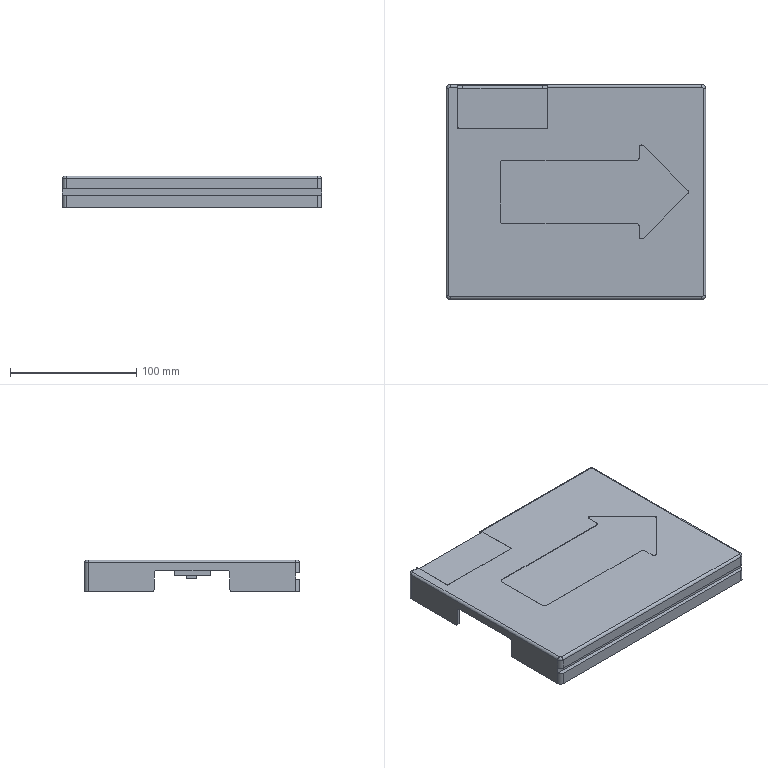NC program | NX | posted with a generic post | part box 205 x 170 x 25 mm
Lines 1 to 1975 of 3445:
N10 G17 G21 G94 G90
(FLOOR_WALL , TOOL : D63)
N12 T03 M6
N14 G54
N16 G17 G0 G90 X-140.5 Y88.497 B0. C0. S6500 M3
N18 G43 Z30. H3
N20 Z3.
N22 G94 G1 Z0. F1250.
N24 X-137.5
N26 X137.5
N28 Y50.548
N30 X-137.5
N32 Y12.599
N34 X137.5
N36 Y-25.351
N38 X-137.5
N40 Y-63.3
N42 X137.5
N44 X140.5
N46 Z3.
N48 G0 Z30.
N50 M5
(ADAPTIVE_MILLING , TOOL : D10)
N52 T04 M6
N54 G54
N56 G17 G0 G90 X-113.707 Y-0.06 B0. C0. S9500 M3
N58 G43 Z30. H4
N60 Z-11.5
N62 G94 G1 Z-12.5 F1000.
N64 X-112.926 Y-0.34 F3000.
N66 X-112.138 Y-0.596
N68 G3 X-111.06 Y-0.06 R1.017
N70 X-110.299 Y3.003 R8.28
N72 X-110.016 Y12.871 R111.643
N74 G1 X-110.012 Y15.121
N76 X-110.009 Y18.996
N78 X-110.008 Y32.621
N80 Y85.371
N82 X-110.007 Y85.496
N84 X-110.005 Y85.621
N86 G2 X-107.512 Y89.901 R5.714
N88 X-102.071 Y91.964 R12.309
N90 X-93.343 Y92.458 R61.608
N92 G1 X-92.218 Y92.467
N94 X-90.593 Y92.475
N96 X-88.843 Y92.481
N98 X-85.843 Y92.484
N100 X-79.468 Y92.486
N102 X103.032
N104 X103.157 Y92.484
N106 X103.282 Y92.478
N108 X103.406 Y92.467
N110 G2 X107.568 Y89.756 R5.951
N112 X109.527 Y84.141 R13.051
N114 X109.958 Y75.783 R67.595
N116 G1 X109.967 Y74.658
N118 X109.974 Y73.283
N120 X109.98 Y71.408
N122 X109.984 Y68.533
N124 X109.986 Y62.783
N126 Y1.283
N128 X109.989 Y0.658
N130 X109.992 Y-1.092
N132 Y-2.717
N134 X109.991 Y-3.217
N136 X109.993 Y-3.842
N138 X109.994 Y-5.217
N140 X109.993 Y-6.092
N142 X109.995 Y-6.842
N144 Y-7.717
N146 X109.994 Y-8.342
N148 X109.997 Y-9.467
N150 X109.995 Y-10.342
N152 X109.997 Y-11.466
N154 X109.996 Y-12.341
N156 X109.999 Y-13.716
N158 X109.997 Y-14.466
N160 X109.998 Y-15.341
N162 Y-15.716
N164 X109.995 Y-17.091
N166 X109.997 Y-17.716
N168 X109.996 Y-19.216
N170 X109.995 Y-19.841
N172 X109.997 Y-20.841
N174 X109.995 Y-22.091
N176 X109.996 Y-22.716
N178 X109.995 Y-24.216
N180 X109.994 Y-24.841
N182 X109.997 Y-25.841
N184 X109.994 Y-27.091
N186 X109.996 Y-27.716
N188 X109.995 Y-29.216
N190 X109.994 Y-29.841
N192 X109.997 Y-30.841
N194 X109.994 Y-32.216
N196 X109.997 Y-33.341
N198 X109.996 Y-34.091
N200 X109.997 Y-34.966
N202 X109.998 Y-35.466
N204 X109.996 Y-36.466
N206 X109.997 Y-37.216
N208 X109.996 Y-38.216
N210 X109.995 Y-38.591
N212 X109.997 Y-39.466
N214 X109.995 Y-40.841
N216 X109.997 Y-41.591
N218 X109.996 Y-42.466
N220 X109.995 Y-42.841
N222 X109.998 Y-44.091
N224 X109.996 Y-44.841
N226 X109.998 Y-46.091
N228 X109.995 Y-47.341
N230 X109.997 Y-48.091
N232 X109.996 Y-48.966
N234 X109.995 Y-49.466
N236 X109.997 Y-50.341
N238 X109.995 Y-51.716
N240 X109.996 Y-52.466
N242 Y-53.341
N244 X109.995 Y-53.716
N246 X109.998 Y-54.966
N248 X109.996 Y-55.716
N250 X109.998 Y-56.966
N252 X109.995 Y-58.216
N254 X109.997 Y-58.841
N256 X109.995 Y-60.216
N258 X109.994 Y-60.966
N260 X109.996 Y-61.591
N262 X109.995 Y-62.966
N264 X109.994 Y-63.716
N266 X109.996 Y-64.591
N268 X109.995 Y-65.716
N270 X109.997 Y-66.591
N272 X109.995 Y-67.966
N274 X109.997 Y-68.841
N276 X109.995 Y-70.091
N278 X109.998 Y-71.341
N280 X109.997 Y-71.966
N282 X109.998 Y-73.466
N284 X109.999 Y-73.966
N286 X109.996 Y-74.966
N288 X109.999 Y-76.216
N290 X109.996 Y-77.466
N292 X109.999 Y-78.716
N294 X109.996 Y-79.841
N296 X109.997 Y-80.466
N298 X109.996 Y-81.841
N300 G2 X109.952 Y-86.089 R74.037
N302 X107.109 Y-90.171 R6.086
N304 X101.34 Y-92.069 R13.643
N306 X92.23 Y-92.467 R79.25
N308 G1 X90.98 Y-92.474
N310 X89.105 Y-92.48
N312 X86.355 Y-92.484
N314 X80.98 Y-92.486
N316 X22.23
N318 X21.48 Y-92.49
N320 X20.355 Y-92.492
N322 X19.48
N324 X18.73 Y-92.494
N326 X17.605
N328 X17.23
N330 X16.355 Y-92.496
N332 X15.355 Y-92.495
N334 X14.855 Y-92.494
N336 X14.23 Y-92.496
N338 X12.855 Y-92.495
N340 X12.23 Y-92.494
N342 X11.23 Y-92.497
N344 X9.855 Y-92.494
N346 X8.73 Y-92.498
N348 X7.855 Y-92.496
N350 X6.48 Y-92.499
N352 X5.48 Y-92.496
N354 X4.23 Y-92.499
N356 X3.48 Y-92.497
N358 X2.605 Y-92.498
N360 X2.105 Y-92.499
N362 X1.105 Y-92.497
N364 X0.23 Y-92.498
N366 X-1.27 Y-92.495
N368 X-2.02 Y-92.497
N370 X-3.02 Y-92.496
N372 X-3.645
N374 X-4.27 Y-92.498
N376 X-5.27 Y-92.496
N378 X-6.02 Y-92.497
N380 X-7.145 Y-92.496
N382 X-7.52 Y-92.495
N384 X-8.52 Y-92.498
N386 X-9.52 Y-92.496
N388 X-10.395 Y-92.498
N390 X-11.395 Y-92.496
N392 X-11.895 Y-92.495
N394 X-12.645 Y-92.497
N396 X-13.645 Y-92.496
N398 X-14.27
N400 X-14.77 Y-92.497
N402 X-15.895 Y-92.496
N404 X-17.145 Y-92.498
N406 X-18.02 Y-92.497
N408 X-19.395 Y-92.499
N410 X-20.395 Y-92.497
N412 X-21.145 Y-92.498
N414 X-22.27 Y-92.497
N416 X-22.645 Y-92.496
N418 X-23.77 Y-92.498
N420 X-25.02 Y-92.496
N422 X-25.77 Y-92.497
N424 X-26.77 Y-92.496
N426 X-27.27 Y-92.495
N428 X-28.02 Y-92.497
N430 X-29.145 Y-92.496
N432 X-29.77
N434 X-30.645 Y-92.498
N436 X-31.52 Y-92.496
N438 X-32.895 Y-92.499
N440 X-33.895 Y-92.497
N442 X-35.145 Y-92.499
N444 X-35.895 Y-92.498
N446 X-36.77
N448 X-37.27 Y-92.499
N450 X-38.27 Y-92.497
N452 X-39.145 Y-92.498
N454 X-40.52 Y-92.496
N456 X-41.52 Y-92.498
N458 X-42.895 Y-92.495
N460 X-44.02 Y-92.498
N462 X-44.77 Y-92.497
N464 X-46.02 Y-92.498
N466 X-46.895 Y-92.497
N468 X-47.895 Y-92.498
N470 X-49.27 Y-92.495
N472 X-49.895 Y-92.497
N474 X-51.395 Y-92.496
N476 X-52.27 Y-92.494
N478 X-53.145 Y-92.497
N480 X-54.395 Y-92.495
N482 X-55.145 Y-92.497
N484 X-56.27 Y-92.496
N486 X-56.645 Y-92.495
N488 X-57.52 Y-92.497
N490 X-58.52 Y-92.496
N492 X-59.145 Y-92.494
N494 X-59.77 Y-92.496
N496 X-61.27
N498 X-62.02 Y-92.494
N500 X-63.02 Y-92.497
N502 X-64.395 Y-92.494
N504 X-65.52 Y-92.498
N506 X-66.395 Y-92.496
N508 X-67.77 Y-92.499
N510 X-68.77 Y-92.496
N512 X-69.52 Y-92.498
N514 X-70.645 Y-92.496
N516 X-71.02
N518 X-72.145 Y-92.498
N520 X-73.395 Y-92.496
N522 X-74.02 Y-92.497
N524 X-75.52 Y-92.496
N526 X-76.27 Y-92.494
N528 X-77.145 Y-92.497
N530 X-78.395 Y-92.495
N532 X-79.145 Y-92.497
N534 X-80.27 Y-92.496
N536 X-80.645 Y-92.495
N538 X-81.52 Y-92.497
N540 X-82.895 Y-92.495
N542 X-83.77 Y-92.497
N544 X-85.02 Y-92.495
N546 X-86.27 Y-92.498
N548 X-87.02 Y-92.497
N550 X-88.02 Y-92.498
N552 X-88.395 Y-92.499
N554 X-89.52 Y-92.496
N556 X-90.645 Y-92.499
N558 X-91.52 Y-92.497
N560 X-92.77 Y-92.499
N562 X-94.145 Y-92.496
N564 X-94.77 Y-92.497
N566 X-96.27 Y-92.496
N568 X-97.145 Y-92.495
N570 X-98.145 Y-92.497
N572 X-99.395 Y-92.495
N574 X-100.27 Y-92.497
N576 X-101.27 Y-92.496
N578 X-101.645 Y-92.495
N580 X-102.77 Y-92.498
N582 X-103.02
N584 X-103.145 Y-92.495
N586 X-103.27 Y-92.489
N588 X-103.394 Y-92.478
N590 G2 X-107.561 Y-89.775 R5.946
N592 X-109.522 Y-84.161 R13.072
N594 X-109.964 Y-75.053 R72.527
N596 G1 X-109.972 Y-73.678
N598 X-109.978 Y-71.928
N600 X-109.983 Y-69.303
N602 X-109.985 Y-64.553
N604 X-109.986 Y-9.553
N606 Y-3.803
N608 G2 X-109.488 Y1.421 R59.156
N610 G3 X-109.035 Y13.657 R126.191
N612 G1 X-109.028 Y15.532
N614 X-109.023 Y18.032
N616 X-109.02 Y22.032
N618 X-109.018 Y33.532
N620 Y82.407
N622 X-109.017 Y82.532
N624 G2 X-105.313 Y88.837 R7.659
N626 X-99.211 Y90.928 R15.285
N628 X-90.358 Y91.436 R67.62
N630 G1 X-89.233 Y91.448
N632 X-87.858 Y91.458
N634 X-86.358 Y91.465
N636 X-84.233 Y91.47
N638 X-80.983 Y91.474
N640 X-73.608 Y91.476
N642 X26.392
N644 X27.142 Y91.479
N646 X28.267 Y91.481
N648 X29.142
N650 X29.892 Y91.483
N652 X31.017
N654 X31.392
N656 X32.267 Y91.485
N658 X33.267 Y91.484
N660 X33.767 Y91.483
N662 X34.392 Y91.485
N664 X35.767 Y91.484
N666 X36.392
N668 X37.392 Y91.486
N670 X38.767 Y91.484
N672 X39.892 Y91.487
N674 X40.767 Y91.485
N676 X42.142 Y91.488
N678 X43.142 Y91.486
N680 X44.392 Y91.488
N682 X45.142 Y91.487
N684 X46.017
N686 X46.517 Y91.488
N688 X47.517 Y91.486
N690 X48.392 Y91.488
N692 X49.892 Y91.485
N694 X50.642 Y91.486
N696 X51.517
N698 X52.142 Y91.484
N700 X53.517 Y91.488
N702 X54.767 Y91.485
N704 X55.892 Y91.488
N706 X56.517 Y91.486
N708 X57.892 Y91.488
N710 X58.767 Y91.489
N712 X59.517 Y91.487
N714 X60.517 Y91.488
N716 X61.017 Y91.489
N718 X61.767 Y91.487
N720 X62.892 Y91.488
N722 X63.517
N724 X64.392 Y91.486
N726 X65.267 Y91.488
N728 X66.642 Y91.485
N730 X67.642 Y91.487
N732 X68.892 Y91.485
N734 X69.642 Y91.486
N736 X70.517 Y91.485
N738 X71.017
N740 X72.017 Y91.487
N742 X72.892 Y91.485
N744 X74.267 Y91.488
N746 X75.267 Y91.486
N748 X76.517 Y91.488
N750 X77.267 Y91.487
N752 X78.142
N754 X78.642 Y91.488
N756 X79.642 Y91.486
N758 X80.392 Y91.487
N760 X81.392 Y91.486
N762 X81.892 Y91.485
N764 X82.642 Y91.486
N766 X83.767 Y91.485
N768 X84.267 Y91.484
N770 X85.517 Y91.487
N772 X86.267 Y91.486
N774 X87.517 Y91.488
N776 X88.392 Y91.486
N778 X89.517 Y91.488
N780 X90.642 Y91.485
N782 X91.767 Y91.488
N784 X92.767 Y91.486
N786 X94.017 Y91.488
N788 X94.767 Y91.486
N790 X95.642 Y91.487
N792 X96.267 Y91.489
N794 X97.517 Y91.486
N796 X98.392 Y91.487
N798 G2 X101.748 Y91.258 R13.333
N800 X106.894 Y86.824 R8.296
N802 X108.602 Y80.333 R18.54
N804 X108.957 Y70.343 R106.668
N806 G1 X108.965 Y68.593
N808 X108.97 Y66.468
N810 X108.974 Y63.093
N812 X108.975 Y55.218
N814 Y4.218
N816 X108.98 Y3.343
N818 X108.983 Y2.218
N820 Y1.468
N822 X108.986 Y0.843
N824 X108.987 Y-0.407
N826 Y-1.407
N828 X108.989 Y-2.032
N830 X108.99 Y-3.407
N832 Y-4.157
N834 X108.993 Y-5.032
N836 X108.992 Y-6.032
N838 X108.994 Y-6.907
N840 Y-8.032
N842 X108.996 Y-9.157
N844 X108.995 Y-9.907
N846 X108.997 Y-11.032
N848 X108.998 Y-11.407
N850 X108.996 Y-12.532
N852 X108.998 Y-13.407
N854 X108.995 Y-14.657
N856 X108.998 Y-15.907
N858 X108.995 Y-17.032
N860 X108.998 Y-18.282
N862 X108.995 Y-19.407
N864 X108.997 Y-20.657
N866 X108.995 Y-21.782
N868 X108.998 Y-23.157
N870 X108.995 Y-24.157
N872 X108.997 Y-25.407
N874 X108.995 Y-26.282
N876 X108.996 Y-27.032
N878 X108.999 Y-28.032
N880 X108.995 Y-29.282
N882 X108.998 Y-30.407
N884 X108.995 Y-31.657
N886 X108.998 Y-32.782
N888 X108.995 Y-34.032
N890 X108.998 Y-35.031
N892 X108.996 Y-35.906
N894 X108.997 Y-36.906
N896 Y-37.531
N898 X108.996 Y-38.156
N900 X108.998 Y-39.406
N902 X108.996 Y-40.156
N904 X108.997 Y-41.281
N906 X108.998 Y-41.781
N908 X108.996 Y-42.656
N910 X108.999 Y-43.906
N912 X108.997 Y-44.656
N914 X108.998 Y-45.906
N916 Y-46.406
N918 X108.996 Y-47.281
N920 X108.997 Y-48.156
N922 X108.995 Y-49.406
N924 X108.997 Y-50.406
N926 X108.996 Y-51.156
N928 X108.997 Y-52.281
N930 X108.998 Y-52.656
N932 X108.996 Y-53.406
N934 X108.998 Y-54.656
N936 X108.996 Y-55.656
N938 X108.998 Y-56.906
N940 X108.994 Y-58.281
N942 X108.997 Y-59.531
N944 X108.994 Y-60.781
N946 X108.996 Y-61.906
N948 X108.994 Y-63.156
N950 X108.995 Y-63.906
N952 Y-65.156
N954 X108.994 Y-65.781
N956 X108.996 Y-66.656
N958 X108.994 Y-67.656
N960 X108.997 Y-68.656
N962 X108.995 Y-69.656
N964 X108.997 Y-70.656
N966 Y-71.281
N968 X108.995 Y-72.031
N970 X108.999 Y-73.406
N972 X108.996 Y-74.656
N974 X108.999 Y-75.906
N976 X108.996 Y-77.156
N978 X108.997 Y-77.906
N980 X108.996 Y-79.156
N982 X108.994 Y-79.781
N984 X108.997 Y-81.031
N986 G2 X108.729 Y-84.383 R12.051
N988 X104.319 Y-89.4 R8.335
N990 X97.827 Y-91.106 R18.539
N992 X87.587 Y-91.459 R113.672
N994 G1 X85.837 Y-91.466
N996 X83.337 Y-91.471
N998 X79.462 Y-91.474
N1000 X67.962 Y-91.476
N1002 X25.212
N1004 X24.337 Y-91.48
N1006 X23.212 Y-91.483
N1008 X22.337
N1010 X21.587 Y-91.487
N1012 X20.462 Y-91.489
N1014 X19.462 Y-91.488
N1016 X18.587 Y-91.492
N1018 X17.837
N1020 X17.337 Y-91.491
N1022 X16.087 Y-91.495
N1024 X14.837 Y-91.493
N1026 X13.962 Y-91.495
N1028 X12.962 Y-91.494
N1030 X12.462 Y-91.493
N1032 X11.462 Y-91.496
N1034 X10.212 Y-91.494
N1036 X9.087 Y-91.497
N1038 X7.837 Y-91.495
N1040 X7.087 Y-91.497
N1042 X5.837
N1044 X5.087 Y-91.496
N1046 X4.462 Y-91.497
N1048 X3.212
N1050 X2.587 Y-91.496
N1052 X1.837 Y-91.497
N1054 X0.712 Y-91.495
N1056 X-0.163 Y-91.497
N1058 X-1.163 Y-91.496
N1060 X-2.038 Y-91.497
N1062 X-3.288 Y-91.495
N1064 X-4.163 Y-91.497
N1066 X-5.163 Y-91.495
N1068 X-6.038 Y-91.497
N1070 X-7.038 Y-91.496
N1072 X-7.413 Y-91.495
N1074 X-8.413 Y-91.497
N1076 X-9.163 Y-91.496
N1078 X-10.413 Y-91.497
N1080 X-10.913 Y-91.498
N1082 X-11.788 Y-91.496
N1084 X-12.663 Y-91.497
N1086 X-13.788 Y-91.496
N1088 X-14.788 Y-91.498
N1090 X-15.663 Y-91.496
N1092 X-16.413 Y-91.497
N1094 X-16.913 Y-91.499
N1096 X-17.913 Y-91.497
N1098 X-19.038 Y-91.499
N1100 X-20.288 Y-91.496
N1102 X-21.163 Y-91.498
N1104 X-22.038 Y-91.497
N1106 X-22.413 Y-91.496
N1108 X-23.663 Y-91.498
N1110 X-24.663 Y-91.496
N1112 X-25.913 Y-91.498
N1114 X-26.663 Y-91.497
N1116 X-27.913
N1118 X-28.413 Y-91.498
N1120 X-29.288 Y-91.497
N1122 X-30.413 Y-91.499
N1124 X-31.538 Y-91.497
N1126 X-32.663 Y-91.499
N1128 X-33.538 Y-91.498
N1130 X-34.538 Y-91.499
N1132 X-35.163
N1134 X-35.788 Y-91.497
N1136 X-36.788 Y-91.499
N1138 X-37.788 Y-91.497
N1140 X-38.413 Y-91.498
N1142 X-39.163 Y-91.499
N1144 X-40.038 Y-91.497
N1146 X-41.038 Y-91.498
N1148 X-41.538 Y-91.499
N1150 X-42.663 Y-91.496
N1152 X-43.413 Y-91.498
N1154 X-44.538 Y-91.497
N1156 X-45.038 Y-91.496
N1158 X-45.788 Y-91.497
N1160 X-46.538 Y-91.496
N1162 X-47.163 Y-91.495
N1164 X-48.413 Y-91.498
N1166 X-49.538 Y-91.495
N1168 X-50.663 Y-91.497
N1170 X-51.913 Y-91.495
N1172 X-53.163 Y-91.497
N1174 X-54.038 Y-91.495
N1176 X-55.163 Y-91.497
N1178 X-56.163 Y-91.495
N1180 X-56.913 Y-91.496
N1182 X-57.538 Y-91.498
N1184 X-58.913 Y-91.494
N1186 X-60.288 Y-91.498
N1188 X-61.538 Y-91.494
N1190 X-62.788 Y-91.498
N1192 X-63.788 Y-91.496
N1194 X-64.413 Y-91.497
N1196 X-65.038 Y-91.498
N1198 X-66.288 Y-91.496
N1200 X-67.413 Y-91.498
N1202 X-68.288 Y-91.497
N1204 X-69.413
N1206 X-70.038 Y-91.499
N1208 X-70.913 Y-91.497
N1210 X-72.038 Y-91.498
N1212 X-73.413 Y-91.495
N1214 X-74.413 Y-91.497
N1216 X-75.663 Y-91.494
N1218 X-76.913 Y-91.497
N1220 X-77.788 Y-91.495
N1222 X-78.663 Y-91.496
N1224 X-79.163 Y-91.498
N1226 X-80.163 Y-91.495
N1228 X-81.538 Y-91.498
N1230 X-82.413 Y-91.496
N1232 X-83.663 Y-91.497
N1234 X-84.663 Y-91.499
N1236 X-85.663 Y-91.497
N1238 X-86.288 Y-91.498
N1240 X-87.663 Y-91.496
N1242 X-88.663 Y-91.494
N1244 X-89.788 Y-91.498
N1246 G2 X-100.661 Y-91.46 R403.061
N1248 X-106.405 Y-87.682 R7.741
N1250 X-108.484 Y-81.314 R15.886
N1252 X-108.943 Y-72.206 R76.882
N1254 G1 X-108.953 Y-70.956
N1256 X-108.961 Y-69.456
N1258 X-108.967 Y-67.581
N1260 X-108.972 Y-64.581
N1262 X-108.975 Y-59.456
N1264 Y-6.206
N1266 X-108.973 Y-5.831
N1268 X-108.968 Y-5.456
N1270 X-108.965 Y-5.331
N1272 X-108.955 Y-4.956
N1274 G2 X-108.323 Y3.645 R431.319
N1276 G3 X-108.034 Y20.14 R313.133
N1278 G1 X-108.031 Y24.39
N1280 X-108.029 Y35.265
N1282 Y79.39
N1284 X-108.027 Y79.765
N1286 X-108.021 Y80.14
N1288 X-108.018 Y80.265
N1290 G2 X-107.545 Y83.002 R10.279
N1292 X-107.008 Y85.159 R7.662
N1294 X-102.587 Y89.537 R8.454
N1296 X-98.749 Y90.168 R10.273
N1298 X-78.253 Y90.463 R461.789
N1300 G1 X-70.128 Y90.465
N1302 X23.372
N1304 X24.247 Y90.47
N1306 X25.372 Y90.472
N1308 X26.247 Y90.473
N1310 X26.997 Y90.476
N1312 X28.122 Y90.478
N1314 X29.122
N1316 X29.872 Y90.48
N1318 X30.872 Y90.481
N1320 X31.372 Y90.48
N1322 X32.247 Y90.483
N1324 X33.247 Y90.482
N1326 X33.872
N1328 X34.747 Y90.485
N1330 X35.997 Y90.483
N1332 X37.247 Y90.486
N1334 X37.997 Y90.485
N1336 X39.247 Y90.487
N1338 X39.872 Y90.488
N1340 X40.747 Y90.486
N1342 X41.997 Y90.488
N1344 X42.747 Y90.487
N1346 X43.872 Y90.488
N1348 X44.247 Y90.489
N1350 X45.247 Y90.486
N1352 X45.997 Y90.488
N1354 X47.122 Y90.486
N1356 X47.497 Y90.485
N1358 X48.372 Y90.487
N1360 X49.497 Y90.485
N1362 X50.497 Y90.487
N1364 X51.497 Y90.485
N1366 X51.997 Y90.484
N1368 X53.122 Y90.487
N1370 X54.247 Y90.485
N1372 X55.122 Y90.487
N1374 X55.997 Y90.486
N1376 X56.622 Y90.485
N1378 X58.122 Y90.489
N1380 X59.122 Y90.487
N1382 X60.372 Y90.49
N1384 X61.372 Y90.487
N1386 X62.497 Y90.489
N1388 X63.872 Y90.485
N1390 X64.747 Y90.487
N1392 X65.747 Y90.486
N1394 X66.122 Y90.485
N1396 X67.372 Y90.487
N1398 X68.247 Y90.485
N1400 X69.247 Y90.487
N1402 X69.622
N1404 X70.497 Y90.486
N1406 X71.247 Y90.487
N1408 X71.747 Y90.488
N1410 X72.872 Y90.485
N1412 X73.747 Y90.487
N1414 X74.747 Y90.486
N1416 X75.122
N1418 X75.997 Y90.487
N1420 X76.747
N1422 X77.247 Y90.486
N1424 X78.122 Y90.487
N1426 X79.247 Y90.485
N1428 X80.372 Y90.487
N1430 X81.622 Y90.484
N1432 X82.747 Y90.487
N1434 X83.997 Y90.485
N1436 X84.997 Y90.487
N1438 X85.747 Y90.486
N1440 X86.872 Y90.487
N1442 X87.372 Y90.488
N1444 X88.372 Y90.486
N1446 G2 X98.37 Y90.439 R289.105
N1448 X100.293 Y90.072 R11.936
N1450 X102.683 Y89.498 R8.118
N1452 X107.047 Y85.063 R8.454
N1454 X107.664 Y81.349 R10.118
N1456 X107.963 Y60.603 R451.059
N1458 G1 X107.964 Y51.978
N1460 X107.965 Y7.228
N1462 X107.971 Y6.103
N1464 X107.972 Y5.103
N1466 X107.973 Y4.353
N1468 X107.977 Y3.478
N1470 X107.979 Y2.478
N1472 Y1.478
N1474 X107.983 Y0.603
N1476 Y-0.397
N1478 Y-1.272
N1480 X107.987 Y-2.147
N1482 Y-3.147
N1484 Y-3.647
N1486 X107.99 Y-4.397
N1488 Y-5.522
N1490 Y-6.022
N1492 X107.993 Y-6.772
N1494 Y-7.772
N1496 X107.992 Y-8.147
N1498 X107.995 Y-9.022
N1500 X107.994 Y-10.022
N1502 X107.997 Y-11.272
N1504 X107.996 Y-12.022
N1506 X107.997 Y-13.272
N1508 X107.998 Y-13.772
N1510 X107.996 Y-14.522
N1512 X107.997 Y-15.647
N1514 X107.998 Y-16.147
N1516 X107.996 Y-17.022
N1518 X107.997 Y-17.772
N1520 X107.998 Y-18.397
N1522 X107.996 Y-19.397
N1524 X107.998 Y-20.522
N1526 X107.996 Y-21.522
N1528 X107.998 Y-22.772
N1530 X107.995 Y-24.022
N1532 X107.998 Y-25.147
N1534 X107.997 Y-25.772
N1536 X107.995 Y-26.397
N1538 X107.997 Y-27.397
N1540 X107.996 Y-28.147
N1542 X107.994 Y-28.772
N1544 X107.997 Y-30.022
N1546 X107.995 Y-31.272
N1548 X107.997 Y-32.147
N1550 X107.996 Y-33.022
N1552 X107.995 Y-33.397
N1554 X107.998 Y-34.647
N1556 X107.996 Y-35.647
N1558 X107.998 Y-36.772
N1560 X107.997 Y-37.647
N1562 X107.998 Y-38.647
N1564 Y-39.272
N1566 X107.996 Y-40.147
N1568 X107.998 Y-41.272
N1570 X107.996 Y-42.397
N1572 X107.999 Y-43.646
N1574 X107.997 Y-44.521
N1576 X107.998 Y-45.521
N1578 X107.999 Y-45.896
N1580 X107.997 Y-46.771
N1582 Y-47.521
N1584 X107.998 Y-48.021
N1586 X107.996 Y-48.896
N1588 X107.998 Y-50.021
N1590 X107.996 Y-51.021
N1592 X107.998 Y-51.896
N1594 X107.996 Y-52.896
N1596 X107.997 Y-53.646
N1598 X107.998 Y-54.146
N1600 X107.995 Y-55.146
N1602 Y-55.771
N1604 X107.998 Y-56.771
N1606 X107.995 Y-58.021
N1608 X107.997 Y-59.271
N1610 X107.994 Y-60.521
N1612 X107.996 Y-61.396
N1614 X107.995 Y-62.271
N1616 X107.994 Y-62.646
N1618 X107.997 Y-64.021
N1620 X107.995 Y-64.896
N1622 X107.996 Y-65.771
N1624 Y-66.146
N1626 X107.995 Y-67.271
N1628 X107.997 Y-68.271
N1630 X107.995 Y-69.271
N1632 X107.996 Y-70.021
N1634 X107.998 Y-70.646
N1636 X107.995 Y-72.021
N1638 X107.998 Y-73.021
N1640 X107.996 Y-74.021
N1642 X107.995 Y-74.396
N1644 G2 X107.934 Y-81.02 R119.491
N1646 X107.551 Y-82.876 R11.918
N1648 G1 X107.405 Y-83.954
N1650 X107.377 Y-84.068
N1652 G2 X105.839 Y-87.113 R9.315
N1654 X103.186 Y-89.262 R9.325
N1656 X100.542 Y-90.081 R10.061
N1658 X79.984 Y-90.462 R388.023
N1660 G1 X74.484 Y-90.464
N1662 X28.234 Y-90.465
N1664 X27.234 Y-90.471
N1666 X26.484 Y-90.472
N1668 X25.234 Y-90.473
N1670 X24.359 Y-90.478
N1672 X23.359 Y-90.479
N1674 X22.359 Y-90.48
N1676 X21.484 Y-90.484
N1678 X20.609 Y-90.485
N1680 X20.234
N1682 X19.484 Y-90.488
N1684 X18.984 Y-90.49
N1686 X17.984 Y-90.489
N1688 X17.484
N1690 X16.734 Y-90.491
N1692 X15.484 Y-90.492
N1694 X14.734 Y-90.491
N1696 X13.734 Y-90.494
N1698 X12.859 Y-90.493
N1700 X11.984 Y-90.494
N1702 X11.609 Y-90.495
N1704 X10.484 Y-90.494
N1706 X9.234 Y-90.497
N1708 X7.984 Y-90.494
N1710 X7.109 Y-90.496
N1712 X5.984 Y-90.495
N1714 X5.484 Y-90.494
N1716 X4.734 Y-90.496
N1718 X3.484 Y-90.495
N1720 X2.984 Y-90.494
N1722 X2.109 Y-90.496
N1724 X1.234 Y-90.495
N1726 X0.109 Y-90.497
N1728 X-0.891 Y-90.495
N1730 X-1.766 Y-90.497
N1732 X-2.891 Y-90.495
N1734 X-3.766 Y-90.497
N1736 X-4.766 Y-90.495
N1738 X-5.141
N1740 X-5.891 Y-90.496
N1742 X-7.016 Y-90.495
N1744 X-7.516 Y-90.494
N1746 X-8.266 Y-90.496
N1748 X-9.391 Y-90.495
N1750 X-9.891
N1752 X-11.141 Y-90.498
N1754 X-11.891 Y-90.496
N1756 X-13.391 Y-90.499
N1758 X-14.891 Y-90.495
N1760 X-16.266 Y-90.499
N1762 X-17.641 Y-90.495
N1764 X-18.641 Y-90.498
N1766 X-19.891 Y-90.495
N1768 X-20.766 Y-90.497
N1770 X-21.766 Y-90.496
N1772 X-22.516
N1774 X-23.266 Y-90.498
N1776 X-24.516 Y-90.496
N1778 X-25.391 Y-90.498
N1780 X-26.641 Y-90.497
N1782 X-27.766 Y-90.499
N1784 X-29.016 Y-90.496
N1786 X-29.891 Y-90.498
N1788 X-31.141 Y-90.497
N1790 X-31.641 Y-90.496
N1792 X-32.516 Y-90.498
N1794 X-33.641 Y-90.497
N1796 X-34.391 Y-90.498
N1798 X-35.391 Y-90.497
N1800 X-35.766 Y-90.496
N1802 X-36.891 Y-90.499
N1804 X-37.641 Y-90.497
N1806 X-38.891 Y-90.498
N1808 X-39.391 Y-90.499
N1810 X-40.141 Y-90.498
N1812 X-41.266 Y-90.499
N1814 X-41.641
N1816 X-42.766 Y-90.496
N1818 X-43.766 Y-90.498
N1820 X-44.516 Y-90.497
N1822 X-45.766
N1824 X-46.266 Y-90.498
N1826 X-47.016 Y-90.496
N1828 X-48.141 Y-90.497
N1830 X-48.641 Y-90.498
N1832 X-49.391 Y-90.496
N1834 X-50.516 Y-90.497
N1836 X-51.016 Y-90.498
N1838 X-51.891 Y-90.496
N1840 X-52.766 Y-90.497
N1842 X-54.016 Y-90.495
N1844 X-55.016 Y-90.497
N1846 X-56.141 Y-90.495
N1848 X-57.141 Y-90.497
N1850 X-57.766
N1852 X-58.641 Y-90.495
N1854 X-59.641 Y-90.497
N1856 X-60.141 Y-90.498
N1858 X-61.266 Y-90.495
N1860 X-62.266 Y-90.498
N1862 X-63.266 Y-90.496
N1864 X-63.891
N1866 X-64.641 Y-90.498
N1868 X-65.766 Y-90.496
N1870 X-67.141 Y-90.499
N1872 X-68.141 Y-90.497
N1874 X-69.141 Y-90.499
N1876 X-70.266 Y-90.496
N1878 X-70.891
N1880 X-71.766 Y-90.498
N1882 X-72.891 Y-90.495
N1884 X-74.266 Y-90.498
N1886 X-75.516 Y-90.495
N1888 X-76.641 Y-90.498
N1890 X-77.516 Y-90.496
N1892 X-78.516 Y-90.497
N1894 X-79.266
N1896 X-80.266 Y-90.495
N1898 X-81.016 Y-90.497
N1900 X-82.266 Y-90.496
N1902 X-82.891 Y-90.495
N1904 X-84.016 Y-90.498
N1906 X-85.516 Y-90.494
N1908 X-87.016 Y-90.498
N1910 X-88.265 Y-90.495
N1912 X-89.015 Y-90.496
N1914 X-90.265 Y-90.495
N1916 G2 X-98.389 Y-90.449 R215.992
N1918 X-100.36 Y-90.065 R11.519
N1920 X-102.69 Y-89.494 R8.073
N1922 X-107.056 Y-85.042 R8.455
N1924 X-107.664 Y-81.32 R10.197
N1926 X-107.963 Y-60.574 R454.24
N1928 G1 X-107.964 Y-52.324
N1930 X-107.965 Y-7.949
N1932 X-107.962 Y-7.449
N1934 X-107.956 Y-6.949
N1936 X-107.946 Y-6.449
N1938 G2 X-107.65 Y-1.099 R174.662
N1940 G1 Y81.76
N1942 X-107.648 Y81.806
N1944 X-107.54 Y83.051
N1946 X-107.478 Y83.64
N1948 X-107.252 Y84.402
N1950 X-107.008 Y85.159
N1952 X-106.637 Y85.864
N1954 X-106.249 Y86.56
N1956 X-105.748 Y87.18
N1958 X-105.232 Y87.787
N1960 X-104.62 Y88.297
N1962 X-103.995 Y88.792
N1964 X-103.296 Y89.173
N1966 X-102.587 Y89.537
N1968 X-101.826 Y89.775
N1970 X-101.06 Y89.994
N1972 X-99.499 Y90.15
N1974 X99.499
N1976 X99.553 Y90.147
N1978 X100.299 Y90.072
N1980 X101.162 Y89.974
N1982 X101.925 Y89.745
N1984 X102.683 Y89.498
N1986 X103.387 Y89.125
N1988 X104.082 Y88.734
N1990 X104.7 Y88.231
N1992 X105.305 Y87.713
N1994 X105.813 Y87.1
N1996 X106.306 Y86.474
N1998 X106.685 Y85.773
N2000 X107.047 Y85.063
N2002 X107.283 Y84.302
N2004 X107.499 Y83.535
N2006 X107.65 Y81.974
N2008 X107.648 Y-82.121
N2010 X107.643 Y-82.192
N2012 X107.543 Y-82.935
N2014 X107.472 Y-83.503
N2016 X107.377 Y-84.068
N2018 X106.82 Y-85.571
N2020 X106.346 Y-86.352
N2022 X105.839 Y-87.113
N2024 X104.713 Y-88.257
N2026 X103.96 Y-88.776
N2028 X103.186 Y-89.262
N2030 X101.593 Y-89.874
N2032 X100.542 Y-90.081
N2034 X99.355 Y-90.15
N2036 X-99.499
N2038 X-99.553 Y-90.147
N2040 X-100.423 Y-90.059
N2042 X-101.166 Y-89.973
N2044 X-101.931 Y-89.743
N2046 X-102.69 Y-89.494
N2048 X-103.395 Y-89.12
N2050 X-104.091 Y-88.728
N2052 X-104.71 Y-88.223
N2054 X-105.316 Y-87.703
N2056 X-105.824 Y-87.086
N2058 X-106.317 Y-86.458
N2060 X-106.695 Y-85.754
N2062 X-107.056 Y-85.042
N2064 X-107.289 Y-84.278
N2066 X-107.504 Y-83.509
N2068 X-107.65 Y-81.945
N2070 Y-1.07
N2072 G3 X-108.497 Y-0.073 R1.016
N2074 G1 X-110.074 Y0.185
N2076 Z-9.5
N2078 G0 Z30.
N2080 X-113.709 Y0.063
N2082 Z-24.
N2084 G1 Z-25. F1000.
N2086 X-112.928 Y-0.217 F3000.
N2088 X-112.14 Y-0.473
N2090 G3 X-111.062 Y0.063 R1.017
N2092 X-110.3 Y3.126 R8.28
N2094 X-110.018 Y12.994 R111.643
N2096 G1 X-110.013 Y15.244
N2098 X-110.01 Y19.119
N2100 X-110.009 Y32.744
N2102 Y85.369
N2104 Y85.494
N2106 X-110.007 Y85.619
N2108 G2 X-107.513 Y89.9 R5.714
N2110 X-102.073 Y91.964 R12.307
N2112 X-94.22 Y92.449 R56.36
N2114 G1 X-93.22 Y92.461
N2116 X-91.97 Y92.47
N2118 X-90.345 Y92.478
N2120 X-88.345 Y92.483
N2122 X-85.22 Y92.487
N2124 X-77.72 Y92.488
N2126 X103.03
N2128 X103.155 Y92.486
N2130 X103.279 Y92.48
N2132 X103.404 Y92.469
N2134 G2 X107.569 Y89.764 R5.929
N2136 X109.53 Y84.149 R13.127
N2138 X109.967 Y74.916 R74.185
N2140 G1 X109.975 Y73.541
N2142 X109.981 Y71.666
N2144 X109.985 Y68.916
N2146 X109.987 Y63.541
N2148 X109.988 Y-83.709
N2150 X109.991 Y-84.334
N2152 G2 X109.713 Y-87.051 R7.36
N2154 X105.923 Y-90.842 R7.054
N2156 X99.861 Y-92.227 R17.847
N2158 X88.992 Y-92.482 R150.153
N2160 G1 X86.242 Y-92.486
N2162 X80.617 Y-92.488
N2164 X10.992
N2166 X10.242 Y-92.492
N2168 X9.117 Y-92.494
N2170 X8.242
N2172 X7.492 Y-92.496
N2174 X6.367
N2176 X5.992 Y-92.495
N2178 X5.117 Y-92.498
N2180 X4.117 Y-92.496
N2182 X3.617
N2184 X2.992 Y-92.497
N2186 X1.617
N2188 X0.992 Y-92.496
N2190 X-0.008 Y-92.499
N2192 X-1.383 Y-92.496
N2194 X-2.383 Y-92.499
N2196 X-3.508 Y-92.497
N2198 X-4.508 Y-92.499
N2200 X-5.258 Y-92.498
N2202 X-6.383 Y-92.5
N2204 X-7.008 Y-92.501
N2206 X-7.883 Y-92.499
N2208 X-9.133 Y-92.501
N2210 X-10.383 Y-92.498
N2212 X-11.008 Y-92.499
N2214 X-12.508 Y-92.498
N2216 X-13.133 Y-92.497
N2218 X-14.133 Y-92.499
N2220 X-15.383 Y-92.497
N2222 X-16.133 Y-92.499
N2224 X-17.008 Y-92.498
N2226 X-17.508 Y-92.497
N2228 X-18.383 Y-92.499
N2230 X-19.633 Y-92.497
N2232 X-20.883 Y-92.5
N2234 X-21.508 Y-92.499
N2236 X-23.008 Y-92.5
N2238 X-23.633 Y-92.501
N2240 X-24.508 Y-92.499
N2242 X-25.758 Y-92.501
N2244 X-27.133 Y-92.498
N2246 X-28.508 Y-92.501
N2248 X-29.633 Y-92.498
N2250 X-30.383 Y-92.5
N2252 X-31.633 Y-92.498
N2254 X-32.508 Y-92.5
N2256 X-33.508 Y-92.498
N2258 X-34.883 Y-92.501
N2260 X-35.508 Y-92.5
N2262 X-37.008
N2264 X-37.883 Y-92.502
N2266 X-38.633 Y-92.5
N2268 X-39.508 Y-92.501
N2270 X-40.008 Y-92.502
N2272 X-41.008 Y-92.499
N2274 X-41.883 Y-92.501
N2276 X-43.258 Y-92.498
N2278 X-44.258 Y-92.5
N2280 X-45.633 Y-92.497
N2282 X-46.883 Y-92.5
N2284 X-48.258 Y-92.497
N2286 X-49.383 Y-92.5
N2288 X-50.258 Y-92.498
N2290 X-51.508 Y-92.5
N2292 X-52.258 Y-92.499
N2294 X-53.383 Y-92.5
N2296 X-54.008
N2298 X-54.758 Y-92.498
N2300 X-55.883 Y-92.501
N2302 X-56.883 Y-92.498
N2304 X-58.133 Y-92.501
N2306 X-58.883 Y-92.499
N2308 X-59.758 Y-92.5
N2310 X-60.383 Y-92.501
N2312 X-61.758 Y-92.498
N2314 X-63.008 Y-92.501
N2316 X-64.258 Y-92.498
N2318 X-65.633 Y-92.501
N2320 X-66.758 Y-92.498
N2322 X-67.508 Y-92.5
N2324 X-68.758 Y-92.498
N2326 X-69.633 Y-92.5
N2328 X-70.758 Y-92.498
N2330 X-72.008 Y-92.501
N2332 X-72.883 Y-92.499
N2334 X-74.258 Y-92.501
N2336 X-75.133 Y-92.499
N2338 X-76.383 Y-92.501
N2340 X-77.633 Y-92.498
N2342 X-78.383 Y-92.5
N2344 X-79.383 Y-92.498
N2346 X-79.883 Y-92.497
N2348 X-80.758 Y-92.499
N2350 X-81.758 Y-92.498
N2352 X-82.633 Y-92.5
N2354 X-83.633 Y-92.498
N2356 X-84.508 Y-92.5
N2358 X-85.633 Y-92.498
N2360 X-86.758 Y-92.5
N2362 X-87.883 Y-92.498
N2364 X-88.758 Y-92.5
N2366 G2 X-103.506 Y-92.468 R720.01
N2368 X-107.763 Y-89.476 R6.126
N2370 X-109.574 Y-83.806 R13.863
N2372 X-109.972 Y-74.195 R84.004
N2374 G1 X-109.979 Y-72.57
N2376 X-109.984 Y-70.32
N2378 X-109.987 Y-66.695
N2380 X-109.988 Y-55.695
N2382 Y-3.695
N2384 X-109.987 Y-3.57
N2386 G2 X-109.478 Y1.653 R63.436
N2388 G3 X-109.036 Y14.14 R132.847
N2390 G1 X-109.029 Y16.14
N2392 X-109.024 Y18.89
N2394 X-109.021 Y23.64
N2396 X-109.02 Y46.765
N2398 Y82.39
N2400 X-109.019 Y82.515
N2402 G2 X-105.327 Y88.827 R7.655
N2404 X-98.857 Y90.982 R15.595
N2406 X-88.75 Y91.454 R85.166
N2408 G1 X-87.375 Y91.462
N2410 X-85.625 Y91.469
N2412 X-83.125 Y91.474
N2414 X-78.875 Y91.477
N2416 X-63.125 Y91.478
N2418 X99.875
N2420 G2 X106.251 Y87.911 R7.579
N2422 X108.409 Y81.835 R14.85
N2424 X108.944 Y72.233 R70.54
N2426 G1 X108.955 Y70.983
N2428 X108.963 Y69.483
N2430 X108.97 Y67.483
N2432 X108.974 Y64.733
N2434 X108.977 Y59.608
N2436 Y-28.392
N2438 Y-80.767
N2440 X108.981 Y-81.642
N2442 X108.984 Y-82.392
N2444 X108.983 Y-82.517
N2446 X108.981 Y-82.642
N2448 G2 X105.301 Y-88.83 R7.627
N2450 X99.078 Y-90.947 R15.393
N2452 X90.348 Y-91.438 R68.829
N2454 G1 X89.223 Y-91.45
N2456 X87.848 Y-91.459
N2458 X86.098 Y-91.467
N2460 X83.848 Y-91.472
N2462 X80.348 Y-91.476
N2464 X71.598 Y-91.477
N2466 X13.973 Y-91.478
N2468 X13.098 Y-91.482
N2470 X11.973 Y-91.485
N2472 X11.098
N2474 X10.348 Y-91.489
N2476 X9.223 Y-91.49
N2478 X8.223
N2480 X7.348 Y-91.494
N2482 X6.598
N2484 X6.098 Y-91.493
N2486 X4.848 Y-91.497
N2488 X3.473 Y-91.494
N2490 X2.598 Y-91.497
N2492 X1.598 Y-91.496
N2494 X1.223 Y-91.495
N2496 X0.223 Y-91.497
N2498 X-0.777 Y-91.496
N2500 X-1.402
N2502 X-2.152 Y-91.498
N2504 X-3.027 Y-91.497
N2506 X-4.027 Y-91.499
N2508 X-4.652 Y-91.5
N2510 X-5.652 Y-91.498
N2512 X-6.652 Y-91.5
N2514 X-7.777 Y-91.498
N2516 X-8.652 Y-91.499
N2518 X-9.652 Y-91.498
N2520 X-10.277 Y-91.496
N2522 X-11.277 Y-91.498
N2524 X-11.902
N2526 X-12.652 Y-91.496
N2528 X-13.402 Y-91.497
N2530 X-14.652
N2532 X-15.152 Y-91.496
N2534 X-16.027 Y-91.498
N2536 X-16.777 Y-91.497
N2538 X-17.277 Y-91.496
N2540 X-18.277 Y-91.498
N2542 X-19.152 Y-91.497
N2544 X-19.527
N2546 X-20.527 Y-91.5
N2548 X-21.777 Y-91.498
N2550 X-23.027 Y-91.501
N2552 X-23.527 Y-91.5
N2554 X-24.402 Y-91.498
N2556 X-25.527 Y-91.5
N2558 X-26.152 Y-91.499
N2560 X-26.777 Y-91.498
N2562 X-28.152 Y-91.501
N2564 X-29.152 Y-91.498
N2566 X-30.152 Y-91.5
N2568 X-31.152 Y-91.498
N2570 X-32.277 Y-91.501
N2572 X-33.027 Y-91.499
N2574 X-34.152 Y-91.501
N2576 X-34.902 Y-91.503
N2578 X-35.902 Y-91.5
N2580 X-37.277 Y-91.503
N2582 X-38.527 Y-91.5
N2584 X-39.527 Y-91.501
N2586 X-40.652 Y-91.499
N2588 X-41.777 Y-91.501
N2590 X-43.027 Y-91.498
N2592 X-44.277 Y-91.5
N2594 X-45.527 Y-91.497
N2596 X-46.777 Y-91.5
N2598 X-47.652 Y-91.498
N2600 X-48.527 Y-91.5
N2602 X-48.902
N2604 X-50.277 Y-91.498
N2606 X-51.277 Y-91.5
N2608 X-52.277 Y-91.498
N2610 X-53.277 Y-91.5
N2612 X-54.152 Y-91.499
N2614 X-54.527 Y-91.498
N2616 X-55.527 Y-91.5
N2618 X-56.777 Y-91.498
N2620 X-57.777 Y-91.5
N2622 X-58.402 Y-91.499
N2624 X-59.152 Y-91.497
N2626 X-60.277 Y-91.5
N2628 X-60.902 Y-91.499
N2630 X-61.402 Y-91.498
N2632 X-62.402 Y-91.5
N2634 X-62.902 Y-91.501
N2636 X-64.027 Y-91.499
N2638 X-65.277 Y-91.501
N2640 X-66.402 Y-91.498
N2642 X-67.402 Y-91.5
N2644 X-68.152 Y-91.499
N2646 X-69.277 Y-91.5
N2648 X-69.777
N2650 X-70.652 Y-91.499
N2652 X-71.652 Y-91.5
N2654 X-72.652 Y-91.499
N2656 X-73.902 Y-91.501
N2658 X-74.902 Y-91.499
N2660 X-75.777 Y-91.5
N2662 X-76.777 Y-91.498
N2664 X-77.402
N2666 X-78.027 Y-91.5
N2668 X-79.027 Y-91.498
N2670 X-80.402 Y-91.501
N2672 X-81.277 Y-91.499
N2674 X-82.402 Y-91.5
N2676 X-83.152 Y-91.499
N2678 X-84.277 Y-91.5
N2680 X-84.902
N2682 X-85.402 Y-91.499
N2684 X-86.652 Y-91.5
N2686 X-87.652 Y-91.498
N2688 G2 X-100.65 Y-91.463 R497.171
N2690 X-106.4 Y-87.695 R7.74
N2692 X-108.498 Y-81.204 R15.925
N2694 X-108.944 Y-72.221 R77.966
N2696 G1 X-108.955 Y-70.971
N2698 X-108.964 Y-69.346
N2700 X-108.97 Y-67.346
N2702 X-108.974 Y-64.471
N2704 X-108.977 Y-59.096
N2706 Y-6.096
N2708 X-108.975 Y-5.721
N2710 X-108.967 Y-5.221
N2712 X-108.957 Y-4.846
N2714 G2 X-108.336 Y3.63 R332.087
N2716 G3 X-108.038 Y19.125 R285.284
N2718 G1 X-108.034 Y22.5
N2720 X-108.031 Y28.875
N2722 Y79.375
N2724 X-108.029 Y79.75
N2726 X-108.023 Y80.125
N2728 X-108.02 Y80.25
N2730 G2 X-107.544 Y83.009 R10.147
N2732 X-107.008 Y85.159 R7.668
N2734 X-102.587 Y89.537 R8.454
N2736 X-98.749 Y90.168 R10.273
N2738 X-75.629 Y90.475 R516.319
N2740 G1 X-74.379 Y90.478
N2742 X-73.629 Y90.477
N2744 X-72.754 Y90.478
N2746 X-72.254 Y90.479
N2748 X-71.254 Y90.477
N2750 X-70.504 Y90.478
N2752 X-69.504 Y90.477
N2754 X-69.004 Y90.476
N2756 X-67.629 Y90.479
N2758 X-66.379 Y90.476
N2760 X-65.129 Y90.479
N2762 X-63.879 Y90.476
N2764 X-62.629 Y90.479
N2766 X-61.504 Y90.476
N2768 X-60.879 Y90.478
N2770 X-59.504 Y90.477
N2772 X-58.879 Y90.475
N2774 X-57.754 Y90.478
N2776 X-56.754 Y90.476
N2778 X-55.379 Y90.479
N2780 X-54.129 Y90.476
N2782 X-52.879 Y90.479
N2784 X-51.754 Y90.476
N2786 X-51.004 Y90.478
N2788 X-50.004 Y90.477
N2790 X-49.629 Y90.476
N2792 X-48.379 Y90.479
N2794 X-47.504 Y90.477
N2796 X-46.254 Y90.479
N2798 X-45.004 Y90.476
N2800 X-44.379 Y90.477
N2802 X-42.879 Y90.476
N2804 X-42.254 Y90.475
N2806 X-41.379 Y90.477
N2808 X-40.254 Y90.476
N2810 X-39.379 Y90.478
N2812 X-38.004 Y90.475
N2814 X-37.129 Y90.478
N2816 X-36.004 Y90.476
N2818 X-35.254 Y90.477
N2820 X-34.004 Y90.476
N2822 X-32.754 Y90.479
N2824 X-32.004 Y90.477
N2826 X-31.129 Y90.478
N2828 X-30.629 Y90.479
N2830 X-29.754 Y90.477
N2832 X-28.379 Y90.48
N2834 X-27.629 Y90.478
N2836 X-26.754 Y90.479
N2838 X-26.254 Y90.48
N2840 X-25.254 Y90.477
N2842 X-24.379 Y90.479
N2844 X-22.879 Y90.476
N2846 X-22.129 Y90.478
N2848 X-21.254 Y90.477
N2850 X-20.629 Y90.475
N2852 X-19.254 Y90.479
N2854 X-18.004 Y90.476
N2856 X-16.879 Y90.479
N2858 X-16.254 Y90.478
N2860 X-14.879 Y90.479
N2862 X-14.004 Y90.48
N2864 X-13.379 Y90.479
N2866 X-12.004
N2868 X-11.129 Y90.481
N2870 X-10.504 Y90.479
N2872 X-9.129 Y90.48
N2874 X-8.379 Y90.481
N2876 X-7.379 Y90.478
N2878 X-6.004 Y90.48
N2880 X-4.754 Y90.477
N2882 X-3.379 Y90.48
N2884 X-2.379 Y90.477
N2886 X-1.254 Y90.479
N2888 X-0.379 Y90.477
N2890 X0.871 Y90.479
N2892 X1.996 Y90.477
N2894 X2.871 Y90.479
N2896 X4.121 Y90.476
N2898 X5.371 Y90.479
N2900 X5.996 Y90.478
N2902 X7.496 Y90.479
N2904 X8.246 Y90.48
N2906 X8.996 Y90.478
N2908 X9.871 Y90.479
N2910 X10.371 Y90.48
N2912 X11.371 Y90.478
N2914 X12.121 Y90.479
N2916 X13.121 Y90.477
N2918 X13.496
N2920 X14.496 Y90.479
N2922 X15.246 Y90.477
N2924 X16.246 Y90.478
N2926 X16.871 Y90.48
N2928 X17.871 Y90.477
N2930 X19.246 Y90.48
N2932 X20.371 Y90.477
N2934 X21.121 Y90.478
N2936 X21.996 Y90.477
N2938 X22.496 Y90.476
N2940 X23.371 Y90.478
N2942 X24.621 Y90.476
N2944 X25.996 Y90.479
N2946 X27.121 Y90.476
N2948 X27.746 Y90.478
N2950 X29.121 Y90.477
N2952 X29.746 Y90.475
N2954 X30.871 Y90.478
N2956 X31.871 Y90.476
N2958 X33.121 Y90.479
N2960 X33.871 Y90.477
N2962 X35.121 Y90.479
N2964 X36.371 Y90.476
N2966 X37.121 Y90.478
N2968 X37.996 Y90.477
N2970 X38.496 Y90.476
N2972 X39.371 Y90.478
N2974 X40.746 Y90.475
N2976 X41.496 Y90.477
N2978 X42.371 Y90.476
N2980 X42.871
N2982 X43.871 Y90.478
N2984 X44.746 Y90.476
N2986 X46.246 Y90.479
N2988 X46.996 Y90.478
N2990 X47.871
N2992 X48.371 Y90.479
N2994 X49.246 Y90.477
N2996 X50.496 Y90.479
N2998 X51.746 Y90.476
N3000 X52.371 Y90.478
N3002 X53.871 Y90.476
N3004 X54.496 Y90.475
N3006 X55.371 Y90.477
N3008 X56.621 Y90.475
N3010 X57.871 Y90.479
N3012 X58.496 Y90.477
N3014 X59.996 Y90.479
N3016 X60.621 Y90.48
N3018 X61.496 Y90.478
N3020 X62.621 Y90.479
N3022 X63.496 Y90.477
N3024 X64.871 Y90.48
N3026 X65.871 Y90.477
N3028 X67.121 Y90.48
N3030 X67.871 Y90.478
N3032 X68.746 Y90.479
N3034 X69.371 Y90.48
N3036 X70.621 Y90.477
N3038 X71.246 Y90.478
N3040 X72.746 Y90.477
N3042 X73.371 Y90.475
N3044 X74.246 Y90.478
N3046 X75.371 Y90.476
N3048 X76.246 Y90.478
N3050 X77.621 Y90.475
N3052 X78.621 Y90.478
N3054 X79.871 Y90.476
N3056 X80.621 Y90.477
N3058 X81.496
N3060 X82.121 Y90.475
N3062 X83.371 Y90.478
N3064 X83.996 Y90.477
N3066 X85.496 Y90.479
N3068 X86.121 Y90.48
N3070 X86.996 Y90.478
N3072 X88.121 Y90.479
N3074 X88.996 Y90.477
N3076 X90.371 Y90.48
N3078 G2 X98.37 Y90.433 R232.099
N3080 X100.271 Y90.074 R11.902
N3082 X102.683 Y89.498 R8.137
N3084 X107.047 Y85.063 R8.454
N3086 X107.668 Y81.224 R10.35
N3088 X107.965 Y60.103 R456.57
N3090 G1 X107.966 Y50.103
N3092 Y5.353
N3094 X107.97 Y4.603
N3096 X107.972 Y3.478
N3098 Y2.603
N3100 X107.974 Y1.853
N3102 Y0.728
N3104 X107.973 Y0.353
N3106 X107.976 Y-0.522
N3108 X107.975 Y-1.522
N3110 X107.974 Y-2.022
N3112 X107.975 Y-2.647
N3114 Y-4.022
N3116 X107.974 Y-4.647
N3118 X107.977 Y-5.647
N3120 X107.974 Y-7.022
N3122 X107.978 Y-8.147
N3124 X107.976 Y-9.022
N3126 X107.979 Y-10.397
N3128 X107.976 Y-11.397
N3130 X107.979 Y-12.647
N3132 X107.977 Y-13.397
N3134 X107.978 Y-14.272
N3136 X107.979 Y-14.772
N3138 X107.977 Y-15.772
N3140 X107.978 Y-16.647
N3142 X107.975 Y-18.147
N3144 X107.977 Y-18.897
N3146 X107.976 Y-19.897
N3148 Y-20.522
N3150 X107.978 Y-21.147
N3152 X107.976 Y-22.147
N3154 X107.977 Y-22.897
N3156 X107.976 Y-24.022
N3158 X107.975 Y-24.397
N3160 X107.978 Y-25.397
N3162 X107.976 Y-26.397
N3164 X107.978 Y-27.272
N3166 X107.976 Y-28.272
N3168 X107.975 Y-28.772
N3170 X107.977 Y-29.522
N3172 X107.976 Y-30.522
N3174 Y-31.147
N3176 X107.977 Y-31.647
N3178 X107.976 Y-32.772
N3180 X107.978 Y-34.022
N3182 X107.976 Y-34.897
N3184 X107.979 Y-36.271
N3186 X107.977 Y-37.271
N3188 X107.978 Y-38.021
N3190 X107.976 Y-39.146
N3192 Y-39.521
N3194 X107.978 Y-40.646
N3196 X107.975 Y-41.896
N3198 X107.977 Y-42.646
N3200 X107.976 Y-43.646
N3202 X107.975 Y-44.146
N3204 X107.977 Y-44.896
N3206 X107.975 Y-46.021
N3208 X107.976 Y-46.646
N3210 X107.978 Y-47.521
N3212 X107.976 Y-48.396
N3214 X107.979 Y-49.771
N3216 X107.977 Y-50.771
N3218 X107.979 Y-52.021
N3220 X107.977 Y-52.771
N3222 X107.978 Y-53.646
N3224 X107.979 Y-54.146
N3226 X107.977 Y-55.146
N3228 X107.978 Y-56.021
N3230 X107.976 Y-57.396
N3232 X107.978 Y-58.396
N3234 X107.975 Y-59.771
N3236 X107.978 Y-60.896
N3238 X107.976 Y-61.646
N3240 X107.978 Y-62.896
N3242 X107.977 Y-63.771
N3244 X107.978 Y-64.771
N3246 X107.975 Y-66.146
N3248 X107.976 Y-66.771
N3250 Y-68.271
N3252 X107.974 Y-69.146
N3254 X107.977 Y-70.021
N3256 X107.975 Y-71.271
N3258 X107.977 Y-72.021
N3260 X107.976 Y-73.146
N3262 X107.975 Y-73.521
N3264 X107.977 Y-74.396
N3266 X107.975 Y-75.396
N3268 X107.974 Y-76.021
N3270 X107.976 Y-76.646
N3272 X107.975 Y-78.146
N3274 Y-78.521
N3276 G2 X107.62 Y-82.614 R13.785
N3278 G1 X107.377 Y-84.068
N3280 G2 X105.839 Y-87.113 R9.315
N3282 X103.186 Y-89.262 R9.325
N3284 X100.542 Y-90.081 R10.061
N3286 X80.359 Y-90.463 R374.023
N3288 G1 X75.234 Y-90.466
N3290 X49.109 Y-90.467
N3292 X23.734
N3294 X22.109 Y-90.474
N3296 X20.734 Y-90.473
N3298 X19.734 Y-90.476
N3300 X18.234 Y-90.474
N3302 X17.359 Y-90.476
N3304 X16.359
N3306 X14.984 Y-90.481
N3308 X13.734 Y-90.48
N3310 X12.359 Y-90.486
N3312 X11.109 Y-90.485
N3314 X9.859 Y-90.49
N3316 X8.484 Y-90.489
N3318 X7.609 Y-90.492
N3320 X6.734
N3322 X6.234 Y-90.491
N3324 X4.984 Y-90.495
N3326 X3.734 Y-90.493
N3328 X2.484 Y-90.497
N3330 X1.359 Y-90.495
N3332 X0.484 Y-90.497
N3334 X-0.766 Y-90.496
N3336 X-1.766 Y-90.499
N3338 X-3.016 Y-90.496
N3340 X-4.141 Y-90.499
N3342 X-5.391 Y-90.497
N3344 X-6.391 Y-90.499
N3346 X-7.641 Y-90.496
N3348 X-8.641 Y-90.498
N3350 X-9.266 Y-90.497
N3352 X-9.891 Y-90.496
N3354 X-11.016 Y-90.498
N3356 X-12.141 Y-90.496
N3358 X-13.516 Y-90.499
N3360 X-14.641 Y-90.496
N3362 X-15.391 Y-90.498
N3364 X-16.641 Y-90.497
N3366 X-17.266 Y-90.496
N3368 X-18.266 Y-90.498
N3370 X-19.141 Y-90.497
N3372 X-20.391 Y-90.499
N3374 X-21.141 Y-90.498
N3376 X-21.641 Y-90.497
N3378 X-22.266 Y-90.498
N3380 X-22.891 Y-90.5
N3382 X-24.266 Y-90.497
N3384 X-25.641 Y-90.501
N3386 X-26.641 Y-90.498
N3388 X-27.641 Y-90.5
N3390 X-28.766 Y-90.498
N3392 X-29.641 Y-90.5
N3394 X-30.641 Y-90.499
N3396 X-31.016 Y-90.498
N3398 X-32.266 Y-90.502
N3400 X-33.516 Y-90.499
N3402 X-34.391 Y-90.501
N3404 X-35.391 Y-90.5
N3406 X-35.891 Y-90.499
N3408 X-36.891 Y-90.501
N3410 X-37.891 Y-90.499
N3412 X-38.516
N3414 X-39.391 Y-90.501
N3416 X-40.516 Y-90.498
N3418 X-41.516 Y-90.5
N3420 X-42.516 Y-90.499
N3422 X-43.141 Y-90.497
N3424 X-44.266 Y-90.5
N3426 X-45.266 Y-90.498
N3428 X-46.64 Y-90.501
N3430 X-47.765 Y-90.498
N3432 X-48.64 Y-90.5
N3434 X-49.89 Y-90.498
N3436 X-50.89 Y-90.5
N3438 X-51.89 Y-90.498
N3440 X-53.14 Y-90.501
N3442 X-54.015 Y-90.499
N3444 X-55.265 Y-90.5
N3446 X-56.265 Y-90.498
N3448 X-57.265 Y-90.5
N3450 X-57.64 Y-90.501
N3452 X-59.015 Y-90.497
N3454 X-59.89 Y-90.5
N3456 X-60.89 Y-90.499
N3458 X-61.39 Y-90.498
N3460 X-62.64 Y-90.501
N3462 X-63.89 Y-90.498
N3464 X-64.64 Y-90.499
N3466 X-65.89
N3468 X-66.515 Y-90.498
N3470 X-67.515 Y-90.5
N3472 X-68.515 Y-90.498
N3474 X-69.515 Y-90.5
N3476 X-70.515 Y-90.498
N3478 X-71.64 Y-90.501
N3480 X-72.765 Y-90.499
N3482 X-73.64 Y-90.5
N3484 X-74.89 Y-90.498
N3486 X-75.89 Y-90.5
N3488 X-76.765 Y-90.498
N3490 X-78.015 Y-90.501
N3492 X-78.765 Y-90.499
N3494 X-79.89 Y-90.5
N3496 X-80.39 Y-90.501
N3498 X-81.265 Y-90.499
N3500 X-82.265 Y-90.501
N3502 X-83.265 Y-90.499
N3504 X-84.015 Y-90.5
N3506 X-85.14 Y-90.499
N3508 X-85.515 Y-90.498
N3510 X-86.515 Y-90.5
N3512 X-87.39 Y-90.498
N3514 X-88.64 Y-90.5
N3516 X-89.89 Y-90.498
N3518 X-91.015 Y-90.501
N3520 X-92.39 Y-90.498
N3522 X-93.515 Y-90.501
N3524 X-94.89 Y-90.499
N3526 X-95.89 Y-90.501
N3528 G2 X-99.866 Y-90.202 R15.587
N3530 G3 X-101.166 Y-89.973 R6.348
N3532 G2 X-106.317 Y-86.458 R8.456
N3534 X-107.65 Y-81.82 R8.799
N3536 X-107.964 Y-63.449 R386.279
N3538 G1 X-107.966 Y-57.574
N3540 X-107.967 Y-56.699
N3542 X-107.97 Y-56.074
N3544 X-107.972 Y-54.949
N3546 X-107.971 Y-53.574
N3548 X-107.974 Y-52.699
N3550 Y-52.074
N3552 X-107.973 Y-51.449
N3554 X-107.977 Y-50.199
N3556 X-107.975 Y-49.324
N3558 X-107.978 Y-47.949
N3560 X-107.976 Y-46.824
N3562 X-107.978 Y-45.699
N3564 X-107.976 Y-44.574
N3566 X-107.978 Y-43.449
N3568 X-107.976 Y-42.324
N3570 X-107.978 Y-41.199
N3572 X-107.976 Y-40.074
N3574 X-107.978 Y-38.949
N3576 X-107.976 Y-37.824
N3578 X-107.978 Y-36.824
N3580 X-107.975 Y-35.574
N3582 X-107.977 Y-34.699
N3584 X-107.975 Y-33.449
N3586 X-107.977 Y-32.574
N3588 X-107.976 Y-31.824
N3590 X-107.975 Y-31.324
N3592 X-107.978 Y-30.199
N3594 X-107.975 Y-28.949
N3596 X-107.977 Y-28.074
N3598 X-107.975 Y-26.824
N3600 X-107.977 Y-25.949
N3602 X-107.976 Y-25.199
N3604 X-107.975 Y-24.699
N3606 X-107.978 Y-23.574
N3608 X-107.975 Y-22.324
N3610 X-107.977 Y-21.449
N3612 X-107.975 Y-20.199
N3614 X-107.977 Y-19.324
N3616 X-107.976 Y-18.574
N3618 X-107.975 Y-18.074
N3620 X-107.978 Y-16.949
N3622 X-107.975 Y-15.699
N3624 X-107.977 Y-14.824
N3626 G2 X-107.868 Y-4.201 R217.273
N3628 G1 X-107.824 Y-3.453
N3630 X-107.784 Y-2.829
N3632 X-107.724 Y-1.956
N3634 X-107.65 Y-0.932
N3636 Y81.76
N3638 X-107.648 Y81.806
N3640 X-107.54 Y83.051
N3642 X-107.478 Y83.64
N3644 X-107.252 Y84.402
N3646 X-107.008 Y85.159
N3648 X-106.637 Y85.864
N3650 X-106.249 Y86.56
N3652 X-105.748 Y87.18
N3654 X-105.232 Y87.787
N3656 X-104.62 Y88.297
N3658 X-103.995 Y88.792
N3660 X-103.296 Y89.173
N3662 X-102.587 Y89.537
N3664 X-101.826 Y89.775
N3666 X-101.06 Y89.994
N3668 X-99.499 Y90.15
N3670 X99.499
N3672 X99.553 Y90.147
N3674 X100.299 Y90.072
N3676 X101.162 Y89.974
N3678 X101.925 Y89.745
N3680 X102.683 Y89.498
N3682 X103.387 Y89.125
N3684 X104.082 Y88.734
N3686 X104.7 Y88.231
N3688 X105.305 Y87.713
N3690 X105.813 Y87.1
N3692 X106.306 Y86.474
N3694 X106.685 Y85.773
N3696 X107.047 Y85.063
N3698 X107.283 Y84.302
N3700 X107.499 Y83.535
N3702 X107.65 Y81.974
N3704 X107.648 Y-82.121
N3706 X107.643 Y-82.192
N3708 X107.543 Y-82.935
N3710 X107.472 Y-83.503
N3712 X107.377 Y-84.068
N3714 X106.82 Y-85.571
N3716 X106.346 Y-86.352
N3718 X105.839 Y-87.113
N3720 X104.713 Y-88.257
N3722 X103.96 Y-88.776
N3724 X103.186 Y-89.262
N3726 X101.593 Y-89.874
N3728 X100.542 Y-90.081
N3730 X99.355 Y-90.15
N3732 X-99.499
N3734 X-99.553 Y-90.147
N3736 X-100.423 Y-90.059
N3738 X-101.166 Y-89.973
N3740 X-101.931 Y-89.743
N3742 X-102.69 Y-89.494
N3744 X-103.395 Y-89.12
N3746 X-104.091 Y-88.728
N3748 X-104.71 Y-88.223
N3750 X-105.316 Y-87.703
N3752 X-105.824 Y-87.086
N3754 X-106.317 Y-86.458
N3756 X-106.695 Y-85.754
N3758 X-107.056 Y-85.042
N3760 X-107.289 Y-84.278
N3762 X-107.504 Y-83.509
N3764 X-107.65 Y-81.945
N3766 Y-0.82
N3768 G3 X-108.497 Y0.177 R1.016
N3770 G1 X-110.073 Y0.435
N3772 Z-22.
N3774 G0 Z30.
(FLOOR_WALL_1 , TOOL : D10)
N3776 X25.476 Y-1.4
N3778 Z4.
N3780 G1 X49.24 Z2.755 F1000.
N3782 X51.234 Y-1.575 Z2.65
N3784 X53.209 Y-1.905 Z2.545
N3786 X54.409 Y-2.215 Z2.48
N3788 X56.625 Y0. Z2.316
N3790 X54.409 Y2.215 Z2.151
N3792 X53.209 Y1.905 Z2.086
N3794 X51.234 Y1.575 Z1.982
N3796 X49.24 Y1.4 Z1.877
N3798 X48. Z1.812
N3800 X5.8 Z-0.4
N3802 X-36.4 F2500.
N3804 Y-1.4
N3806 X48.
N3808 G2 X54.409 Y-2.215 R25.6
N3810 G1 X56.625 Y0.
N3812 X54.409 Y2.215
N3814 G2 X48. Y1.4 R25.6
N3816 G1 X5.8
N3818 Y5.9
N3820 X-40.9
N3822 Y-5.9
N3824 X48.
N3826 G2 X55.652 Y-7.336 R21.1
N3828 G1 X62.989 Y0.
N3830 X55.652 Y7.336
N3832 G2 X48. Y5.9 R21.1
N3834 G1 X5.8
N3836 Y12.9
N3838 X-47.9
N3840 Y-12.9
N3842 X48.
N3844 G2 X56.858 Y-16.03 R14.1
N3846 G1 X72.888 Y0.
N3848 X56.858 Y16.03
N3850 G2 X48. Y12.9 R14.1
N3852 G1 X5.8
N3854 Y19.9
N3856 X-54.9
N3858 Y-19.9
N3860 X48.
N3862 G2 X55.1 Y-27. R7.1
N3864 G1 Y-27.688
N3866 X82.788 Y0.
N3868 X55.1 Y27.688
N3870 Y27.
N3872 G2 X48. Y19.9 R7.1
N3874 G1 X5.8
N3876 Z1.1
N3878 G0 Z30.
(FLOOR_WALL_1_COPY , TOOL : D10)
N3880 X-67.095 Y69.1
N3882 Z1.5
N3884 G1 X-41.6 Z0.164 F1000.
N3886 Y73. Z-0.041
N3888 X-58. Z-0.9
N3890 X-74.4 F2500.
N3892 Y69.1
N3894 X-41.6
N3896 Y73.
N3898 X-58.
N3900 Y80.
N3902 X-81.4
N3904 Y62.1
N3906 X-34.6
N3908 Y80.
N3910 X-58.
N3912 Y87.
N3914 X-87.429
N3916 X-88.4
N3918 Y55.1
N3920 X-27.6
N3922 Y87.
N3924 X-58.
N3926 Z0.6
N3928 G0 Z30.
N3930 M5